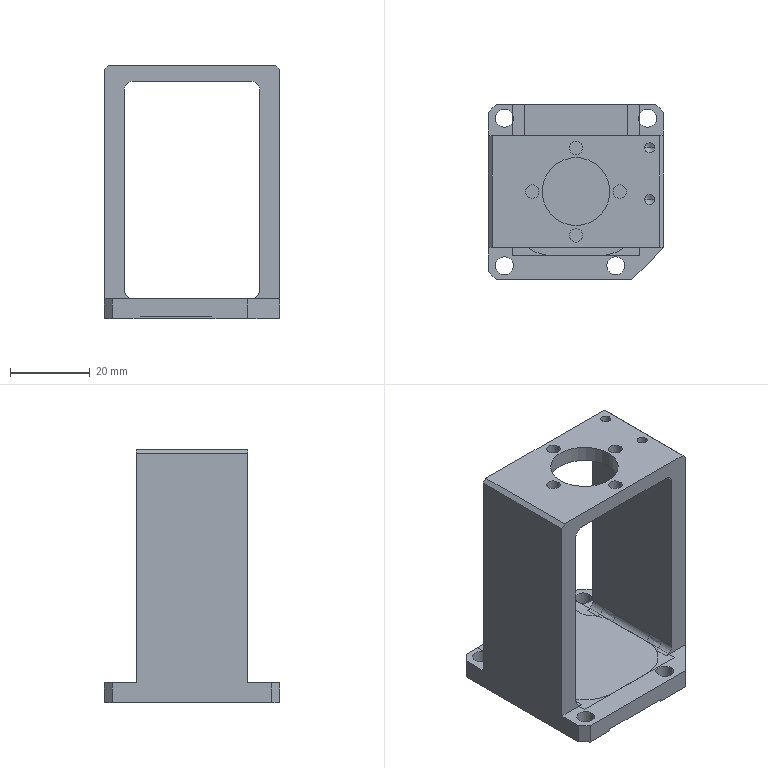NC program | NX | posted with a generic post | part box 44 x 44 x 63.6 mm
Lines 1 to 1841 of 4449:
N10 G17 G21 G94 G90
(CAVITY_MILL_COPY , TOOL : D4)
N12 T04 M6
N14 G54
N16 G17 G0 G90 X-1.665 Y-0.5 B0. C0. S9500 M3
N18 G43 Z30. H4
N20 Z-7.
N22 G94 G1 X11.3 Z-7.679 F1000.
N24 Y0.5 Z-7.732
N26 X0.5 Z-8.298
N28 X-10.3 F2000.
N30 Y-0.5
N32 X11.3
N34 Y0.5
N36 X0.5
N38 Y2.9
N40 X-12.7
N42 Y-2.9
N44 X13.7
N46 Y2.9
N48 X0.5
N50 Y5.3
N52 X-15.1
N54 Y-5.3
N56 X16.1
N58 Y5.3
N60 X0.5
N62 Y7.7
N64 X-17.5
N66 Y-7.7
N68 X18.5
N70 Y7.7
N72 X0.5
N74 Y10.1
N76 X-19.9
N78 Y-10.1
N80 X20.9
N82 Y10.1
N84 X0.5
N86 Y12.5
N88 X-22.3
N90 Y-12.5
N92 X23.3
N94 Y12.5
N96 X0.5
N98 Y14.9
N100 X-24.7 Y14.903
N102 Y-14.9
N104 X25.7
N106 Y14.9
N108 X0.5
N110 Z-7.298
N112 G0 Z30.
N114 X2.665 Y0.5
N116 Z-7.298
N118 G1 X-10.3 Z-7.977 F1000.
N120 Y-0.5 Z-8.03
N122 X0.5 Z-8.596
N124 X11.3 F2000.
N126 Y0.5
N128 X-10.3
N130 Y-0.5
N132 X0.5
N134 Y-2.9
N136 X13.7
N138 Y2.9
N140 X-12.7
N142 Y-2.9
N144 X0.5
N146 Y-5.3
N148 X16.1
N150 Y5.3
N152 X-15.1
N154 Y-5.3
N156 X0.5
N158 Y-7.7
N160 X18.5
N162 Y7.7
N164 X-17.5
N166 Y-7.7
N168 X0.5
N170 Y-10.1
N172 X20.9
N174 Y10.1
N176 X-19.9
N178 Y-10.1
N180 X0.5
N182 Y-12.5
N184 X23.3
N186 Y12.5
N188 X-22.3
N190 Y-12.5
N192 X0.5
N194 Y-14.9
N196 X25.7
N198 Y14.9
N200 X-24.7 Y14.902
N202 Y-14.9
N204 X0.5
N206 Z-7.596
N208 G0 Z30.
N210 X2.665 Y0.5
N212 Z-7.596
N214 G1 X-10.3 Z-8.275 F1000.
N216 Y-0.5 Z-8.328
N218 X0.5 Z-8.894
N220 X11.3 F2000.
N222 Y0.5
N224 X-10.3
N226 Y-0.5
N228 X0.5
N230 Y-2.9
N232 X13.7
N234 Y2.9
N236 X-12.7
N238 Y-2.9
N240 X0.5
N242 Y-5.3
N244 X16.1
N246 Y5.3
N248 X-15.1
N250 Y-5.3
N252 X0.5
N254 Y-7.7
N256 X18.5
N258 Y7.7
N260 X-17.5
N262 Y-7.7
N264 X0.5
N266 Y-10.1
N268 X20.9
N270 Y10.1
N272 X-19.9
N274 Y-10.1
N276 X0.5
N278 Y-12.5
N280 X23.3
N282 Y12.5
N284 X-22.3
N286 Y-12.5
N288 X0.5
N290 Y-14.9
N292 X25.7
N294 Y14.9
N296 X-24.7 Y14.902
N298 Y-14.9
N300 X0.5
N302 Z-7.894
N304 G0 Z30.
N306 X2.665 Y0.5
N308 Z-7.894
N310 G1 X-10.3 Z-8.573 F1000.
N312 Y-0.5 Z-8.625
N314 X0.5 Z-9.191
N316 X11.3 F2000.
N318 Y0.5
N320 X-10.3
N322 Y-0.5
N324 X0.5
N326 Y-2.9
N328 X13.7
N330 Y2.9
N332 X-12.7
N334 Y-2.9
N336 X0.5
N338 Y-5.3
N340 X16.1
N342 Y5.3
N344 X-15.1
N346 Y-5.3
N348 X0.5
N350 Y-7.7
N352 X18.5
N354 Y7.7
N356 X-17.5
N358 Y-7.7
N360 X0.5
N362 Y-10.1
N364 X20.9
N366 Y10.1
N368 X-19.9
N370 Y-10.1
N372 X0.5
N374 Y-12.5
N376 X23.3
N378 Y12.5
N380 X-22.3
N382 Y-12.5
N384 X0.5
N386 Y-14.9
N388 X25.7
N390 Y14.9
N392 X-24.7 Y14.902
N394 Y-14.9
N396 X0.5
N398 Z-8.191
N400 G0 X2.665 Y0.5
N402 G1 X-10.3 Z-8.871 F1000.
N404 Y-0.5 Z-8.923
N406 X0.5 Z-9.489
N408 X11.3 F2000.
N410 Y0.5
N412 X-10.3
N414 Y-0.5
N416 X0.5
N418 Y-2.9
N420 X13.7
N422 Y2.9
N424 X-12.7
N426 Y-2.9
N428 X0.5
N430 Y-5.3
N432 X16.1
N434 Y5.3
N436 X-15.1
N438 Y-5.3
N440 X0.5
N442 Y-7.7
N444 X18.5
N446 Y7.7
N448 X-17.5
N450 Y-7.7
N452 X0.5
N454 Y-10.1
N456 X20.9
N458 Y10.1
N460 X-19.9
N462 Y-10.1
N464 X0.5
N466 Y-12.5
N468 X23.3
N470 Y12.5
N472 X-22.3
N474 Y-12.5
N476 X0.5
N478 Y-14.9
N480 X25.7
N482 Y14.9
N484 X-24.7 Y14.901
N486 Y-14.9
N488 X0.5
N490 Z-8.489
N492 G0 X2.665 Y0.5
N494 G1 X-10.3 Z-9.169 F1000.
N496 Y-0.5 Z-9.221
N498 X0.5 Z-9.787
N500 X11.3 F2000.
N502 Y0.5
N504 X-10.3
N506 Y-0.5
N508 X0.5
N510 Y-2.9
N512 X13.7
N514 Y2.9
N516 X-12.7
N518 Y-2.9
N520 X0.5
N522 Y-5.3
N524 X16.1
N526 Y5.3
N528 X-15.1
N530 Y-5.3
N532 X0.5
N534 Y-7.7
N536 X18.5
N538 Y7.7
N540 X-17.5
N542 Y-7.7
N544 X0.5
N546 Y-10.1
N548 X20.9
N550 Y10.1
N552 X-19.9
N554 Y-10.1
N556 X0.5
N558 Y-12.5
N560 X23.3
N562 Y12.5
N564 X-22.3
N566 Y-12.5
N568 X0.5
N570 Y-14.9
N572 X25.7
N574 Y14.9
N576 X-24.7 Y14.901
N578 Y-14.9
N580 X0.5
N582 Z-8.787
N584 G0 X-1.665 Y-0.5
N586 G1 X11.3 Z-9.467 F1000.
N588 Y0.5 Z-9.519
N590 X0.5 Z-10.085
N592 X-10.3 F2000.
N594 Y-0.5
N596 X11.3
N598 Y0.5
N600 X0.5
N602 Y2.9
N604 X-12.7
N606 Y-2.9
N608 X13.7
N610 Y2.9
N612 X0.5
N614 Y5.3
N616 X-15.1
N618 Y-5.3
N620 X16.1
N622 Y5.3
N624 X0.5
N626 Y7.7
N628 X-17.5
N630 Y-7.7
N632 X18.5
N634 Y7.7
N636 X0.5
N638 Y10.1
N640 X-19.9
N642 Y-10.1
N644 X20.9
N646 Y10.1
N648 X0.5
N650 Y12.5
N652 X-22.3
N654 Y-12.5
N656 X23.3
N658 Y12.5
N660 X0.5
N662 Y14.9
N664 X-24.7
N666 Y-14.9
N668 X25.7
N670 Y14.9
N672 X0.5
N674 Z-9.085
N676 G0 X2.665 Y0.5
N678 G1 X-10.3 Z-9.765 F1000.
N680 Y-0.5 Z-9.817
N682 X0.5 Z-10.383
N684 X11.3 F2000.
N686 Y0.5
N688 X-10.3
N690 Y-0.5
N692 X0.5
N694 Y-2.9
N696 X13.7
N698 Y2.9
N700 X-12.7
N702 Y-2.9
N704 X0.5
N706 Y-5.3
N708 X16.1
N710 Y5.3
N712 X-15.1
N714 Y-5.3
N716 X0.5
N718 Y-7.7
N720 X18.5
N722 Y7.7
N724 X-17.5
N726 Y-7.7
N728 X0.5
N730 Y-10.1
N732 X20.9
N734 Y10.1
N736 X-19.9
N738 Y-10.1
N740 X0.5
N742 Y-12.5
N744 X23.3
N746 Y12.5
N748 X-22.3
N750 Y-12.5
N752 X0.5
N754 Y-14.9
N756 X25.7
N758 Y14.9
N760 X-24.7
N762 Y-14.9
N764 X0.5
N766 Z-9.383
N768 G0 X2.665 Y0.5
N770 G1 X-10.3 Z-10.062 F1000.
N772 Y-0.5 Z-10.115
N774 X0.5 Z-10.681
N776 X11.3 F2000.
N778 Y0.5
N780 X-10.3
N782 Y-0.5
N784 X0.5
N786 Y-2.9
N788 X13.7
N790 Y2.9
N792 X-12.7
N794 Y-2.9
N796 X0.5
N798 Y-5.3
N800 X16.1
N802 Y5.3
N804 X-15.1
N806 Y-5.3
N808 X0.5
N810 Y-7.7
N812 X18.5
N814 Y7.7
N816 X-17.5
N818 Y-7.7
N820 X0.5
N822 Y-10.1
N824 X20.9
N826 Y10.1
N828 X-19.9
N830 Y-10.1
N832 X0.5
N834 Y-12.5
N836 X23.3
N838 Y12.5
N840 X-22.3
N842 Y-12.5
N844 X0.5
N846 Y-14.9
N848 X25.7
N850 Y14.9
N852 X-24.7
N854 Y-14.9
N856 X0.5
N858 Z-9.681
N860 G0 X2.665 Y0.5
N862 G1 X-10.3 Z-10.36 F1000.
N864 Y-0.5 Z-10.413
N866 X0.5 Z-10.979
N868 X11.3 F2000.
N870 Y0.5
N872 X-10.3
N874 Y-0.5
N876 X0.5
N878 Y-2.9
N880 X13.7
N882 Y2.9
N884 X-12.7
N886 Y-2.9
N888 X0.5
N890 Y-5.3
N892 X16.1
N894 Y5.3
N896 X-15.1
N898 Y-5.3
N900 X0.5
N902 Y-7.7
N904 X18.5
N906 Y7.7
N908 X-17.5
N910 Y-7.7
N912 X0.5
N914 Y-10.1
N916 X20.9
N918 Y10.1
N920 X-19.9
N922 Y-10.1
N924 X0.5
N926 Y-12.5
N928 X23.3
N930 Y12.5
N932 X-22.3
N934 Y-12.5
N936 X0.5
N938 Y-14.9
N940 X25.7
N942 Y14.9
N944 X-24.7
N946 Y-14.9
N948 X0.5
N950 Z-9.979
N952 G0 X2.665 Y0.5
N954 G1 X-10.3 Z-10.658 F1000.
N956 Y-0.5 Z-10.711
N958 X0.5 Z-11.277
N960 X11.3 F2000.
N962 Y0.5
N964 X-10.3
N966 Y-0.5
N968 X0.5
N970 Y-2.9
N972 X13.7
N974 Y2.9
N976 X-12.7
N978 Y-2.9
N980 X0.5
N982 Y-5.3
N984 X16.1
N986 Y5.3
N988 X-15.1
N990 Y-5.3
N992 X0.5
N994 Y-7.7
N996 X18.5
N998 Y7.7
N1000 X-17.5
N1002 Y-7.7
N1004 X0.5
N1006 Y-10.1
N1008 X20.9
N1010 Y10.1
N1012 X-19.9
N1014 Y-10.1
N1016 X0.5
N1018 Y-12.5
N1020 X23.3
N1022 Y12.5
N1024 X-22.3
N1026 Y-12.5
N1028 X0.5
N1030 Y-14.9
N1032 X25.7
N1034 Y14.9
N1036 X-24.7
N1038 Y-14.9
N1040 X0.5
N1042 Z-10.277
N1044 G0 X2.665 Y0.5
N1046 G1 X-10.3 Z-10.956 F1000.
N1048 Y-0.5 Z-11.008
N1050 X0.5 Z-11.574
N1052 X11.3 F2000.
N1054 Y0.5
N1056 X-10.3
N1058 Y-0.5
N1060 X0.5
N1062 Y-2.9
N1064 X13.7
N1066 Y2.9
N1068 X-12.7
N1070 Y-2.9
N1072 X0.5
N1074 Y-5.3
N1076 X16.1
N1078 Y5.3
N1080 X-15.1
N1082 Y-5.3
N1084 X0.5
N1086 Y-7.7
N1088 X18.5
N1090 Y7.7
N1092 X-17.5
N1094 Y-7.7
N1096 X0.5
N1098 Y-10.1
N1100 X20.9
N1102 Y10.1
N1104 X-19.9
N1106 Y-10.1
N1108 X0.5
N1110 Y-12.5
N1112 X23.3
N1114 Y12.5
N1116 X-22.3
N1118 Y-12.5
N1120 X0.5
N1122 Y-14.9
N1124 X25.7
N1126 Y14.9
N1128 X-24.7
N1130 Y-14.9
N1132 X0.5
N1134 Z-10.574
N1136 G0 X2.665 Y0.5
N1138 G1 X-10.3 Z-11.254 F1000.
N1140 Y-0.5 Z-11.306
N1142 X0.5 Z-11.872
N1144 X11.3 F2000.
N1146 Y0.5
N1148 X-10.3
N1150 Y-0.5
N1152 X0.5
N1154 Y-2.9
N1156 X13.7
N1158 Y2.9
N1160 X-12.7
N1162 Y-2.9
N1164 X0.5
N1166 Y-5.3
N1168 X16.1
N1170 Y5.3
N1172 X-15.1
N1174 Y-5.3
N1176 X0.5
N1178 Y-7.7
N1180 X18.5
N1182 Y7.7
N1184 X-17.5
N1186 Y-7.7
N1188 X0.5
N1190 Y-10.1
N1192 X20.9
N1194 Y10.1
N1196 X-19.9
N1198 Y-10.1
N1200 X0.5
N1202 Y-12.5
N1204 X23.3
N1206 Y12.5
N1208 X-22.3
N1210 Y-12.5
N1212 X0.5
N1214 Y-14.9
N1216 X25.7
N1218 Y14.9
N1220 X-24.7
N1222 Y-14.9
N1224 X0.5
N1226 Z-10.872
N1228 G0 X2.665 Y0.5
N1230 G1 X-10.3 Z-11.552 F1000.
N1232 Y-0.5 Z-11.604
N1234 X0.5 Z-12.17
N1236 X11.3 F2000.
N1238 Y0.5
N1240 X-10.3
N1242 Y-0.5
N1244 X0.5
N1246 Y-2.9
N1248 X13.7
N1250 Y2.9
N1252 X-12.7
N1254 Y-2.9
N1256 X0.5
N1258 Y-5.3
N1260 X16.1
N1262 Y5.3
N1264 X-15.1
N1266 Y-5.3
N1268 X0.5
N1270 Y-7.7
N1272 X18.5
N1274 Y7.7
N1276 X-17.5
N1278 Y-7.7
N1280 X0.5
N1282 Y-10.1
N1284 X20.9
N1286 Y10.1
N1288 X-19.9
N1290 Y-10.1
N1292 X0.5
N1294 Y-12.5
N1296 X23.3
N1298 Y12.5
N1300 X-22.3
N1302 Y-12.5
N1304 X0.5
N1306 Y-14.9
N1308 X25.7
N1310 Y14.9
N1312 X-24.7
N1314 Y-14.9
N1316 X0.5
N1318 Z-11.17
N1320 G0 X2.665 Y0.5
N1322 G1 X-10.3 Z-11.85 F1000.
N1324 Y-0.5 Z-11.902
N1326 X0.5 Z-12.468
N1328 X11.3 F2000.
N1330 Y0.5
N1332 X-10.3
N1334 Y-0.5
N1336 X0.5
N1338 Y-2.9
N1340 X13.7
N1342 Y2.9
N1344 X-12.7
N1346 Y-2.9
N1348 X0.5
N1350 Y-5.3
N1352 X16.1
N1354 Y5.3
N1356 X-15.1
N1358 Y-5.3
N1360 X0.5
N1362 Y-7.7
N1364 X18.5
N1366 Y7.7
N1368 X-17.5
N1370 Y-7.7
N1372 X0.5
N1374 Y-10.1
N1376 X20.9
N1378 Y10.1
N1380 X-19.9
N1382 Y-10.1
N1384 X0.5
N1386 Y-12.5
N1388 X23.3
N1390 Y12.5
N1392 X-22.3
N1394 Y-12.5
N1396 X0.5
N1398 Y-14.9
N1400 X25.7
N1402 Y14.9
N1404 X-24.7
N1406 Y-14.9
N1408 X0.5
N1410 Z-11.468
N1412 G0 X2.665 Y0.5
N1414 G1 X-10.3 Z-12.148 F1000.
N1416 Y-0.5 Z-12.2
N1418 X0.5 Z-12.766
N1420 X11.3 F2000.
N1422 Y0.5
N1424 X-10.3
N1426 Y-0.5
N1428 X0.5
N1430 Y-2.9
N1432 X13.7
N1434 Y2.9
N1436 X-12.7
N1438 Y-2.9
N1440 X0.5
N1442 Y-5.3
N1444 X16.1
N1446 Y5.3
N1448 X-15.1
N1450 Y-5.3
N1452 X0.5
N1454 Y-7.7
N1456 X18.5
N1458 Y7.7
N1460 X-17.5
N1462 Y-7.7
N1464 X0.5
N1466 Y-10.1
N1468 X20.9
N1470 Y10.1
N1472 X-19.9
N1474 Y-10.1
N1476 X0.5
N1478 Y-12.5
N1480 X23.3
N1482 Y12.5
N1484 X-22.3
N1486 Y-12.5
N1488 X0.5
N1490 Y-14.9
N1492 X25.7
N1494 Y14.9
N1496 X-24.7
N1498 Y-14.9
N1500 X0.5
N1502 Z-11.766
N1504 G0 X2.665 Y0.5
N1506 G1 X-10.3 Z-12.445 F1000.
N1508 Y-0.5 Z-12.498
N1510 X0.5 Z-13.064
N1512 X11.3 F2000.
N1514 Y0.5
N1516 X-10.3
N1518 Y-0.5
N1520 X0.5
N1522 Y-2.9
N1524 X13.7
N1526 Y2.9
N1528 X-12.7
N1530 Y-2.9
N1532 X0.5
N1534 Y-5.3
N1536 X16.1
N1538 Y5.3
N1540 X-15.1
N1542 Y-5.3
N1544 X0.5
N1546 Y-7.7
N1548 X18.5
N1550 Y7.7
N1552 X-17.5
N1554 Y-7.7
N1556 X0.5
N1558 Y-10.1
N1560 X20.9
N1562 Y10.1
N1564 X-19.9
N1566 Y-10.1
N1568 X0.5
N1570 Y-12.5
N1572 X23.3
N1574 Y12.5
N1576 X-22.3
N1578 Y-12.5
N1580 X0.5
N1582 Y-14.9
N1584 X25.7
N1586 Y14.9
N1588 X-24.7
N1590 Y-14.9
N1592 X0.5
N1594 Z-12.064
N1596 G0 X2.665 Y0.5
N1598 G1 X-10.3 Z-12.743 F1000.
N1600 Y-0.5 Z-12.796
N1602 X0.5 Z-13.362
N1604 X11.3 F2000.
N1606 Y0.5
N1608 X-10.3
N1610 Y-0.5
N1612 X0.5
N1614 Y-2.9
N1616 X13.7
N1618 Y2.9
N1620 X-12.7
N1622 Y-2.9
N1624 X0.5
N1626 Y-5.3
N1628 X16.1
N1630 Y5.3
N1632 X-15.1
N1634 Y-5.3
N1636 X0.5
N1638 Y-7.7
N1640 X18.5
N1642 Y7.7
N1644 X-17.5
N1646 Y-7.7
N1648 X0.5
N1650 Y-10.1
N1652 X20.9
N1654 Y10.1
N1656 X-19.9
N1658 Y-10.1
N1660 X0.5
N1662 Y-12.5
N1664 X23.3
N1666 Y12.5
N1668 X-22.3
N1670 Y-12.5
N1672 X0.5
N1674 Y-14.9
N1676 X25.7
N1678 Y14.9
N1680 X-24.7
N1682 Y-14.9
N1684 X0.5
N1686 Z-12.362
N1688 G0 X2.665 Y0.5
N1690 G1 X-10.3 Z-13.041 F1000.
N1692 Y-0.5 Z-13.094
N1694 X0.5 Z-13.66
N1696 X11.3 F2000.
N1698 Y0.5
N1700 X-10.3
N1702 Y-0.5
N1704 X0.5
N1706 Y-2.9
N1708 X13.7
N1710 Y2.9
N1712 X-12.7
N1714 Y-2.9
N1716 X0.5
N1718 Y-5.3
N1720 X16.1
N1722 Y5.3
N1724 X-15.1
N1726 Y-5.3
N1728 X0.5
N1730 Y-7.7
N1732 X18.5
N1734 Y7.7
N1736 X-17.5
N1738 Y-7.7
N1740 X0.5
N1742 Y-10.1
N1744 X20.9
N1746 Y10.1
N1748 X-19.9
N1750 Y-10.1
N1752 X0.5
N1754 Y-12.5
N1756 X23.3
N1758 Y12.5
N1760 X-22.3
N1762 Y-12.5
N1764 X0.5
N1766 Y-14.9
N1768 X25.7
N1770 Y14.9
N1772 X-24.7
N1774 Y-14.9
N1776 X0.5
N1778 Z-12.66
N1780 G0 X2.665 Y0.5
N1782 G1 X-10.3 Z-13.339 F1000.
N1784 Y-0.5 Z-13.391
N1786 X0.5 Z-13.957
N1788 X11.3 F2000.
N1790 Y0.5
N1792 X-10.3
N1794 Y-0.5
N1796 X0.5
N1798 Y-2.9
N1800 X13.7
N1802 Y2.9
N1804 X-12.7
N1806 Y-2.9
N1808 X0.5
N1810 Y-5.3
N1812 X16.1
N1814 Y5.3
N1816 X-15.1
N1818 Y-5.3
N1820 X0.5
N1822 Y-7.7
N1824 X18.5
N1826 Y7.7
N1828 X-17.5
N1830 Y-7.7
N1832 X0.5
N1834 Y-10.1
N1836 X20.9
N1838 Y10.1
N1840 X-19.9
N1842 Y-10.1
N1844 X0.5
N1846 Y-12.5
N1848 X23.3
N1850 Y12.5
N1852 X-22.3
N1854 Y-12.5
N1856 X0.5
N1858 Y-14.9
N1860 X25.7
N1862 Y14.9
N1864 X-24.7
N1866 Y-14.9
N1868 X0.5
N1870 Z-12.957
N1872 G0 X2.665 Y0.5
N1874 G1 X-10.3 Z-13.637 F1000.
N1876 Y-0.5 Z-13.689
N1878 X0.5 Z-14.255
N1880 X11.3 F2000.
N1882 Y0.5
N1884 X-10.3
N1886 Y-0.5
N1888 X0.5
N1890 Y-2.9
N1892 X13.7
N1894 Y2.9
N1896 X-12.7
N1898 Y-2.9
N1900 X0.5
N1902 Y-5.3
N1904 X16.1
N1906 Y5.3
N1908 X-15.1
N1910 Y-5.3
N1912 X0.5
N1914 Y-7.7
N1916 X18.5
N1918 Y7.7
N1920 X-17.5
N1922 Y-7.7
N1924 X0.5
N1926 Y-10.1
N1928 X20.9
N1930 Y10.1
N1932 X-19.9
N1934 Y-10.1
N1936 X0.5
N1938 Y-12.5
N1940 X23.3
N1942 Y12.5
N1944 X-22.3
N1946 Y-12.5
N1948 X0.5
N1950 Y-14.9
N1952 X25.7
N1954 Y14.9
N1956 X-24.7
N1958 Y-14.9
N1960 X0.5
N1962 Z-13.255
N1964 G0 X2.665 Y0.5
N1966 G1 X-10.3 Z-13.935 F1000.
N1968 Y-0.5 Z-13.987
N1970 X0.5 Z-14.553
N1972 X11.3 F2000.
N1974 Y0.5
N1976 X-10.3
N1978 Y-0.5
N1980 X0.5
N1982 Y-2.9
N1984 X13.7
N1986 Y2.9
N1988 X-12.7
N1990 Y-2.9
N1992 X0.5
N1994 Y-5.3
N1996 X16.1
N1998 Y5.3
N2000 X-15.1
N2002 Y-5.3
N2004 X0.5
N2006 Y-7.7
N2008 X18.5
N2010 Y7.7
N2012 X-17.5
N2014 Y-7.7
N2016 X0.5
N2018 Y-10.1
N2020 X20.9
N2022 Y10.1
N2024 X-19.9
N2026 Y-10.1
N2028 X0.5
N2030 Y-12.5
N2032 X23.3
N2034 Y12.5
N2036 X-22.3
N2038 Y-12.5
N2040 X0.5
N2042 Y-14.9
N2044 X25.7
N2046 Y14.9
N2048 X-24.7
N2050 Y-14.9
N2052 X0.5
N2054 Z-13.553
N2056 G0 X2.665 Y0.5
N2058 G1 X-10.3 Z-14.233 F1000.
N2060 Y-0.5 Z-14.285
N2062 X0.5 Z-14.851
N2064 X11.3 F2000.
N2066 Y0.5
N2068 X-10.3
N2070 Y-0.5
N2072 X0.5
N2074 Y-2.9
N2076 X13.7
N2078 Y2.9
N2080 X-12.7
N2082 Y-2.9
N2084 X0.5
N2086 Y-5.3
N2088 X16.1
N2090 Y5.3
N2092 X-15.1
N2094 Y-5.3
N2096 X0.5
N2098 Y-7.7
N2100 X18.5
N2102 Y7.7
N2104 X-17.5
N2106 Y-7.7
N2108 X0.5
N2110 Y-10.1
N2112 X20.9
N2114 Y10.1
N2116 X-19.9
N2118 Y-10.1
N2120 X0.5
N2122 Y-12.5
N2124 X23.3
N2126 Y12.5
N2128 X-22.3
N2130 Y-12.5
N2132 X0.5
N2134 Y-14.9
N2136 X25.7
N2138 Y14.9
N2140 X-24.7
N2142 Y-14.9
N2144 X0.5
N2146 Z-13.851
N2148 G0 X2.665 Y0.5
N2150 G1 X-10.3 Z-14.531 F1000.
N2152 Y-0.5 Z-14.583
N2154 X0.5 Z-15.149
N2156 X11.3 F2000.
N2158 Y0.5
N2160 X-10.3
N2162 Y-0.5
N2164 X0.5
N2166 Y-2.9
N2168 X13.7
N2170 Y2.9
N2172 X-12.7
N2174 Y-2.9
N2176 X0.5
N2178 Y-5.3
N2180 X16.1
N2182 Y5.3
N2184 X-15.1
N2186 Y-5.3
N2188 X0.5
N2190 Y-7.7
N2192 X18.5
N2194 Y7.7
N2196 X-17.5
N2198 Y-7.7
N2200 X0.5
N2202 Y-10.1
N2204 X20.9
N2206 Y10.1
N2208 X-19.9
N2210 Y-10.1
N2212 X0.5
N2214 Y-12.5
N2216 X23.3
N2218 Y12.5
N2220 X-22.3
N2222 Y-12.5
N2224 X0.5
N2226 Y-14.9
N2228 X25.7
N2230 Y14.9
N2232 X-24.7
N2234 Y-14.9
N2236 X0.5
N2238 Z-14.149
N2240 G0 X2.665 Y0.5
N2242 G1 X-10.3 Z-14.828 F1000.
N2244 Y-0.5 Z-14.881
N2246 X0.5 Z-15.447
N2248 X11.3 F2000.
N2250 Y0.5
N2252 X-10.3
N2254 Y-0.5
N2256 X0.5
N2258 Y-2.9
N2260 X13.7
N2262 Y2.9
N2264 X-12.7
N2266 Y-2.9
N2268 X0.5
N2270 Y-5.3
N2272 X16.1
N2274 Y5.3
N2276 X-15.1
N2278 Y-5.3
N2280 X0.5
N2282 Y-7.7
N2284 X18.5
N2286 Y7.7
N2288 X-17.5
N2290 Y-7.7
N2292 X0.5
N2294 Y-10.1
N2296 X20.9
N2298 Y10.1
N2300 X-19.9
N2302 Y-10.1
N2304 X0.5
N2306 Y-12.5
N2308 X23.3
N2310 Y12.5
N2312 X-22.3
N2314 Y-12.5
N2316 X0.5
N2318 Y-14.9
N2320 X25.7
N2322 Y14.9
N2324 X-24.7
N2326 Y-14.9
N2328 X0.5
N2330 Z-14.447
N2332 G0 X2.665 Y0.5
N2334 G1 X-10.3 Z-15.126 F1000.
N2336 Y-0.5 Z-15.179
N2338 X0.5 Z-15.745
N2340 X11.3 F2000.
N2342 Y0.5
N2344 X-10.3
N2346 Y-0.5
N2348 X0.5
N2350 Y-2.9
N2352 X13.7
N2354 Y2.9
N2356 X-12.7
N2358 Y-2.9
N2360 X0.5
N2362 Y-5.3
N2364 X16.1
N2366 Y5.3
N2368 X-15.1
N2370 Y-5.3
N2372 X0.5
N2374 Y-7.7
N2376 X18.5
N2378 Y7.7
N2380 X-17.5
N2382 Y-7.7
N2384 X0.5
N2386 Y-10.1
N2388 X20.9
N2390 Y10.1
N2392 X-19.9
N2394 Y-10.1
N2396 X0.5
N2398 Y-12.5
N2400 X23.3
N2402 Y12.5
N2404 X-22.3
N2406 Y-12.5
N2408 X0.5
N2410 Y-14.9
N2412 X25.7
N2414 Y14.9
N2416 X-24.7
N2418 Y-14.9
N2420 X0.5
N2422 Z-14.745
N2424 G0 X2.665 Y0.5
N2426 G1 X-10.3 Z-15.424 F1000.
N2428 Y-0.5 Z-15.477
N2430 X0.5 Z-16.043
N2432 X11.3 F2000.
N2434 Y0.5
N2436 X-10.3
N2438 Y-0.5
N2440 X0.5
N2442 Y-2.9
N2444 X13.7
N2446 Y2.9
N2448 X-12.7
N2450 Y-2.9
N2452 X0.5
N2454 Y-5.3
N2456 X16.1
N2458 Y5.3
N2460 X-15.1
N2462 Y-5.3
N2464 X0.5
N2466 Y-7.7
N2468 X18.5
N2470 Y7.7
N2472 X-17.5
N2474 Y-7.7
N2476 X0.5
N2478 Y-10.1
N2480 X20.9
N2482 Y10.1
N2484 X-19.9
N2486 Y-10.1
N2488 X0.5
N2490 Y-12.5
N2492 X23.3
N2494 Y12.5
N2496 X-22.3
N2498 Y-12.5
N2500 X0.5
N2502 Y-14.9
N2504 X25.7
N2506 Y14.9
N2508 X-24.7
N2510 Y-14.9
N2512 X0.5
N2514 Z-15.043
N2516 G0 X2.665 Y0.5
N2518 G1 X-10.3 Z-15.722 F1000.
N2520 Y-0.5 Z-15.774
N2522 X0.5 Z-16.34
N2524 X11.3 F2000.
N2526 Y0.5
N2528 X-10.3
N2530 Y-0.5
N2532 X0.5
N2534 Y-2.9
N2536 X13.7
N2538 Y2.9
N2540 X-12.7
N2542 Y-2.9
N2544 X0.5
N2546 Y-5.3
N2548 X16.1
N2550 Y5.3
N2552 X-15.1
N2554 Y-5.3
N2556 X0.5
N2558 Y-7.7
N2560 X18.5
N2562 Y7.7
N2564 X-17.5
N2566 Y-7.7
N2568 X0.5
N2570 Y-10.1
N2572 X20.9
N2574 Y10.1
N2576 X-19.9
N2578 Y-10.1
N2580 X0.5
N2582 Y-12.5
N2584 X23.3
N2586 Y12.5
N2588 X-22.3
N2590 Y-12.5
N2592 X0.5
N2594 Y-14.9
N2596 X25.7
N2598 Y14.9
N2600 X-24.7
N2602 Y-14.9
N2604 X0.5
N2606 Z-15.34
N2608 G0 X2.665 Y0.5
N2610 G1 X-10.3 Z-16.02 F1000.
N2612 Y-0.5 Z-16.072
N2614 X0.5 Z-16.638
N2616 X11.3 F2000.
N2618 Y0.5
N2620 X-10.3
N2622 Y-0.5
N2624 X0.5
N2626 Y-2.9
N2628 X13.7
N2630 Y2.9
N2632 X-12.7
N2634 Y-2.9
N2636 X0.5
N2638 Y-5.3
N2640 X16.1
N2642 Y5.3
N2644 X-15.1
N2646 Y-5.3
N2648 X0.5
N2650 Y-7.7
N2652 X18.5
N2654 Y7.7
N2656 X-17.5
N2658 Y-7.7
N2660 X0.5
N2662 Y-10.1
N2664 X20.9
N2666 Y10.1
N2668 X-19.9
N2670 Y-10.1
N2672 X0.5
N2674 Y-12.5
N2676 X23.3
N2678 Y12.5
N2680 X-22.3
N2682 Y-12.5
N2684 X0.5
N2686 Y-14.9
N2688 X25.7
N2690 Y14.9
N2692 X-24.7
N2694 Y-14.9
N2696 X0.5
N2698 Z-15.638
N2700 G0 X2.665 Y0.5
N2702 G1 X-10.3 Z-16.318 F1000.
N2704 Y-0.5 Z-16.37
N2706 X0.5 Z-16.936
N2708 X11.3 F2000.
N2710 Y0.5
N2712 X-10.3
N2714 Y-0.5
N2716 X0.5
N2718 Y-2.9
N2720 X13.7
N2722 Y2.9
N2724 X-12.7
N2726 Y-2.9
N2728 X0.5
N2730 Y-5.3
N2732 X16.1
N2734 Y5.3
N2736 X-15.1
N2738 Y-5.3
N2740 X0.5
N2742 Y-7.7
N2744 X18.5
N2746 Y7.7
N2748 X-17.5
N2750 Y-7.7
N2752 X0.5
N2754 Y-10.1
N2756 X20.9
N2758 Y10.1
N2760 X-19.9
N2762 Y-10.1
N2764 X0.5
N2766 Y-12.5
N2768 X23.3
N2770 Y12.5
N2772 X-22.3
N2774 Y-12.5
N2776 X0.5
N2778 Y-14.9
N2780 X25.7
N2782 Y14.9
N2784 X-24.7
N2786 Y-14.9
N2788 X0.5
N2790 Z-15.936
N2792 G0 X2.665 Y0.5
N2794 G1 X-10.3 Z-16.616 F1000.
N2796 Y-0.5 Z-16.668
N2798 X0.5 Z-17.234
N2800 X11.3 F2000.
N2802 Y0.5
N2804 X-10.3
N2806 Y-0.5
N2808 X0.5
N2810 Y-2.9
N2812 X13.7
N2814 Y2.9
N2816 X-12.7
N2818 Y-2.9
N2820 X0.5
N2822 Y-5.3
N2824 X16.1
N2826 Y5.3
N2828 X-15.1
N2830 Y-5.3
N2832 X0.5
N2834 Y-7.7
N2836 X18.5
N2838 Y7.7
N2840 X-17.5
N2842 Y-7.7
N2844 X0.5
N2846 Y-10.1
N2848 X20.9
N2850 Y10.1
N2852 X-19.9
N2854 Y-10.1
N2856 X0.5
N2858 Y-12.5
N2860 X23.3
N2862 Y12.5
N2864 X-22.3
N2866 Y-12.5
N2868 X0.5
N2870 Y-14.9
N2872 X25.7
N2874 Y14.9
N2876 X-24.7
N2878 Y-14.9
N2880 X0.5
N2882 Z-16.234
N2884 G0 X2.665 Y0.5
N2886 G1 X-10.3 Z-16.914 F1000.
N2888 Y-0.5 Z-16.966
N2890 X0.5 Z-17.532
N2892 X11.3 F2000.
N2894 Y0.5
N2896 X-10.3
N2898 Y-0.5
N2900 X0.5
N2902 Y-2.9
N2904 X13.7
N2906 Y2.9
N2908 X-12.7
N2910 Y-2.9
N2912 X0.5
N2914 Y-5.3
N2916 X16.1
N2918 Y5.3
N2920 X-15.1
N2922 Y-5.3
N2924 X0.5
N2926 Y-7.7
N2928 X18.5
N2930 Y7.7
N2932 X-17.5
N2934 Y-7.7
N2936 X0.5
N2938 Y-10.1
N2940 X20.9
N2942 Y10.1
N2944 X-19.9
N2946 Y-10.1
N2948 X0.5
N2950 Y-12.5
N2952 X23.3
N2954 Y12.5
N2956 X-22.3
N2958 Y-12.5
N2960 X0.5
N2962 Y-14.9
N2964 X25.7
N2966 Y14.9
N2968 X-24.7
N2970 Y-14.9
N2972 X0.5
N2974 Z-16.532
N2976 G0 X2.665 Y0.5
N2978 G1 X-10.3 Z-17.211 F1000.
N2980 Y-0.5 Z-17.264
N2982 X0.5 Z-17.83
N2984 X11.3 F2000.
N2986 Y0.5
N2988 X-10.3
N2990 Y-0.5
N2992 X0.5
N2994 Y-2.9
N2996 X13.7
N2998 Y2.9
N3000 X-12.7
N3002 Y-2.9
N3004 X0.5
N3006 Y-5.3
N3008 X16.1
N3010 Y5.3
N3012 X-15.1
N3014 Y-5.3
N3016 X0.5
N3018 Y-7.7
N3020 X18.5
N3022 Y7.7
N3024 X-17.5
N3026 Y-7.7
N3028 X0.5
N3030 Y-10.1
N3032 X20.9
N3034 Y10.1
N3036 X-19.9
N3038 Y-10.1
N3040 X0.5
N3042 Y-12.5
N3044 X23.3
N3046 Y12.5
N3048 X-22.3
N3050 Y-12.5
N3052 X0.5
N3054 Y-14.9
N3056 X25.7
N3058 Y14.9
N3060 X-24.7
N3062 Y-14.9
N3064 X0.5
N3066 Z-16.83
N3068 G0 X2.665 Y0.5
N3070 G1 X-10.3 Z-17.509 F1000.
N3072 Y-0.5 Z-17.562
N3074 X0.5 Z-18.128
N3076 X11.3 F2000.
N3078 Y0.5
N3080 X-10.3
N3082 Y-0.5
N3084 X0.5
N3086 Y-2.9
N3088 X13.7
N3090 Y2.9
N3092 X-12.7
N3094 Y-2.9
N3096 X0.5
N3098 Y-5.3
N3100 X16.1
N3102 Y5.3
N3104 X-15.1
N3106 Y-5.3
N3108 X0.5
N3110 Y-7.7
N3112 X18.5
N3114 Y7.7
N3116 X-17.5
N3118 Y-7.7
N3120 X0.5
N3122 Y-10.1
N3124 X20.9
N3126 Y10.1
N3128 X-19.9
N3130 Y-10.1
N3132 X0.5
N3134 Y-12.5
N3136 X23.3
N3138 Y12.5
N3140 X-22.3
N3142 Y-12.5
N3144 X0.5
N3146 Y-14.9
N3148 X25.7
N3150 Y14.9
N3152 X-24.7
N3154 Y-14.9
N3156 X0.5
N3158 Z-17.128
N3160 G0 X2.665 Y0.5
N3162 G1 X-10.3 Z-17.807 F1000.
N3164 Y-0.5 Z-17.86
N3166 X0.5 Z-18.426
N3168 X11.3 F2000.
N3170 Y0.5
N3172 X-10.3
N3174 Y-0.5
N3176 X0.5
N3178 Y-2.9
N3180 X13.7
N3182 Y2.9
N3184 X-12.7
N3186 Y-2.9
N3188 X0.5
N3190 Y-5.3
N3192 X16.1
N3194 Y5.3
N3196 X-15.1
N3198 Y-5.3
N3200 X0.5
N3202 Y-7.7
N3204 X18.5
N3206 Y7.7
N3208 X-17.5
N3210 Y-7.7
N3212 X0.5
N3214 Y-10.1
N3216 X20.9
N3218 Y10.1
N3220 X-19.9
N3222 Y-10.1
N3224 X0.5
N3226 Y-12.5
N3228 X23.3
N3230 Y12.5
N3232 X-22.3
N3234 Y-12.5
N3236 X0.5
N3238 Y-14.9
N3240 X25.7
N3242 Y14.9
N3244 X-24.7
N3246 Y-14.9
N3248 X0.5
N3250 Z-17.426
N3252 G0 X2.665 Y0.5
N3254 G1 X-10.3 Z-18.105 F1000.
N3256 Y-0.5 Z-18.157
N3258 X0.5 Z-18.723
N3260 X11.3 F2000.
N3262 Y0.5
N3264 X-10.3
N3266 Y-0.5
N3268 X0.5
N3270 Y-2.9
N3272 X13.7
N3274 Y2.9
N3276 X-12.7
N3278 Y-2.9
N3280 X0.5
N3282 Y-5.3
N3284 X16.1
N3286 Y5.3
N3288 X-15.1
N3290 Y-5.3
N3292 X0.5
N3294 Y-7.7
N3296 X18.5
N3298 Y7.7
N3300 X-17.5
N3302 Y-7.7
N3304 X0.5
N3306 Y-10.1
N3308 X20.9
N3310 Y10.1
N3312 X-19.9
N3314 Y-10.1
N3316 X0.5
N3318 Y-12.5
N3320 X23.3
N3322 Y12.5
N3324 X-22.3
N3326 Y-12.5
N3328 X0.5
N3330 Y-14.9
N3332 X25.7
N3334 Y14.9
N3336 X-24.7
N3338 Y-14.9
N3340 X0.5
N3342 Z-17.723
N3344 G0 X2.665 Y0.5
N3346 G1 X-10.3 Z-18.403 F1000.
N3348 Y-0.5 Z-18.455
N3350 X0.5 Z-19.021
N3352 X11.3 F2000.
N3354 Y0.5
N3356 X-10.3
N3358 Y-0.5
N3360 X0.5
N3362 Y-2.9
N3364 X13.7
N3366 Y2.9
N3368 X-12.7
N3370 Y-2.9
N3372 X0.5
N3374 Y-5.3
N3376 X16.1
N3378 Y5.3
N3380 X-15.1
N3382 Y-5.3
N3384 X0.5
N3386 Y-7.7
N3388 X18.5
N3390 Y7.7
N3392 X-17.5
N3394 Y-7.7
N3396 X0.5
N3398 Y-10.1
N3400 X20.9
N3402 Y10.1
N3404 X-19.9
N3406 Y-10.1
N3408 X0.5
N3410 Y-12.5
N3412 X23.3
N3414 Y12.5
N3416 X-22.3
N3418 Y-12.5
N3420 X0.5
N3422 Y-14.9
N3424 X25.7
N3426 Y14.9
N3428 X-24.7
N3430 Y-14.9
N3432 X0.5
N3434 Z-18.021
N3436 G0 X2.665 Y0.5
N3438 G1 X-10.3 Z-18.701 F1000.
N3440 Y-0.5 Z-18.753
N3442 X0.5 Z-19.319
N3444 X11.3 F2000.
N3446 Y0.5
N3448 X-10.3
N3450 Y-0.5
N3452 X0.5
N3454 Y-2.9
N3456 X13.7
N3458 Y2.9
N3460 X-12.7
N3462 Y-2.9
N3464 X0.5
N3466 Y-5.3
N3468 X16.1
N3470 Y5.3
N3472 X-15.1
N3474 Y-5.3
N3476 X0.5
N3478 Y-7.7
N3480 X18.5
N3482 Y7.7
N3484 X-17.5
N3486 Y-7.7
N3488 X0.5
N3490 Y-10.1
N3492 X20.9
N3494 Y10.1
N3496 X-19.9
N3498 Y-10.1
N3500 X0.5
N3502 Y-12.5
N3504 X23.3
N3506 Y12.5
N3508 X-22.3
N3510 Y-12.5
N3512 X0.5
N3514 Y-14.9
N3516 X25.7
N3518 Y14.9
N3520 X-24.7
N3522 Y-14.9
N3524 X0.5
N3526 Z-18.319
N3528 G0 X2.665 Y0.5
N3530 G1 X-10.3 Z-18.999 F1000.
N3532 Y-0.5 Z-19.051
N3534 X0.5 Z-19.617
N3536 X11.3 F2000.
N3538 Y0.5
N3540 X-10.3
N3542 Y-0.5
N3544 X0.5
N3546 Y-2.9
N3548 X13.7
N3550 Y2.9
N3552 X-12.7
N3554 Y-2.9
N3556 X0.5
N3558 Y-5.3
N3560 X16.1
N3562 Y5.3
N3564 X-15.1
N3566 Y-5.3
N3568 X0.5
N3570 Y-7.7
N3572 X18.5
N3574 Y7.7
N3576 X-17.5
N3578 Y-7.7
N3580 X0.5
N3582 Y-10.1
N3584 X20.9
N3586 Y10.1
N3588 X-19.9
N3590 Y-10.1
N3592 X0.5
N3594 Y-12.5
N3596 X23.3
N3598 Y12.5
N3600 X-22.3
N3602 Y-12.5
N3604 X0.5
N3606 Y-14.9
N3608 X25.7
N3610 Y14.9
N3612 X-24.7
N3614 Y-14.9
N3616 X0.5
N3618 Z-18.617
N3620 G0 X2.665 Y0.5
N3622 G1 X-10.3 Z-19.296 F1000.
N3624 Y-0.5 Z-19.349
N3626 X0.5 Z-19.915
N3628 X11.3 F2000.
N3630 Y0.5
N3632 X-10.3
N3634 Y-0.5
N3636 X0.5
N3638 Y-2.9
N3640 X13.7
N3642 Y2.9
N3644 X-12.7
N3646 Y-2.9
N3648 X0.5
N3650 Y-5.3
N3652 X16.1
N3654 Y5.3
N3656 X-15.1
N3658 Y-5.3
N3660 X0.5
N3662 Y-7.7
N3664 X18.5
N3666 Y7.7
N3668 X-17.5
N3670 Y-7.7
N3672 X0.5
N3674 Y-10.1
N3676 X20.9
N3678 Y10.1
N3680 X-19.9